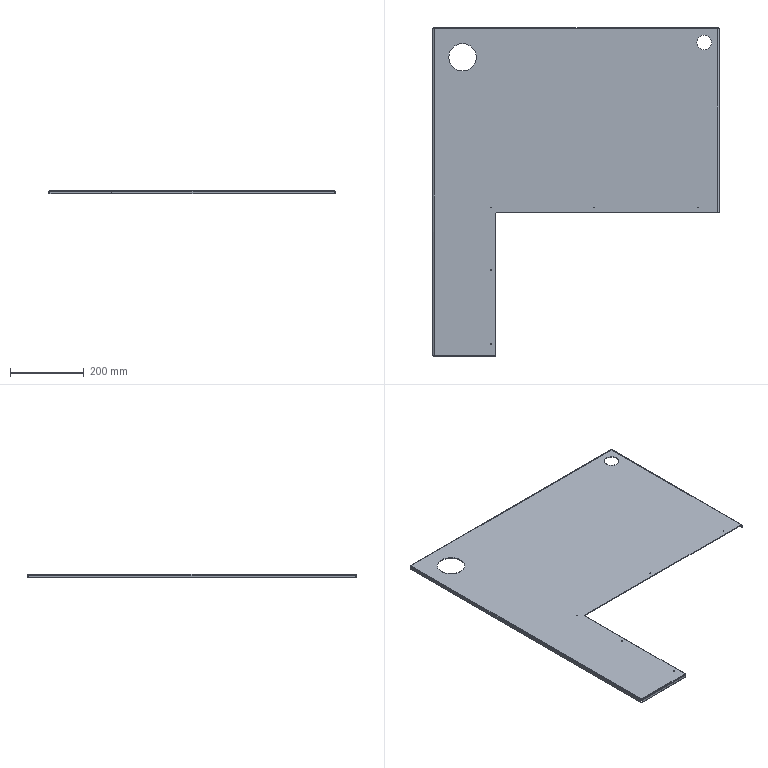Part | STEP file | 11-FG-JX01511 | 1 solid | 55 faces | box 775 x 890 x 10 mm | volume 929885 mm3 | plane 26 | cylinder 23 | spline 6 | commonest cylinder face diameters 2.5 x10 1.473 x4 5.473 x4 40 x2 74.689 x2 10 x1